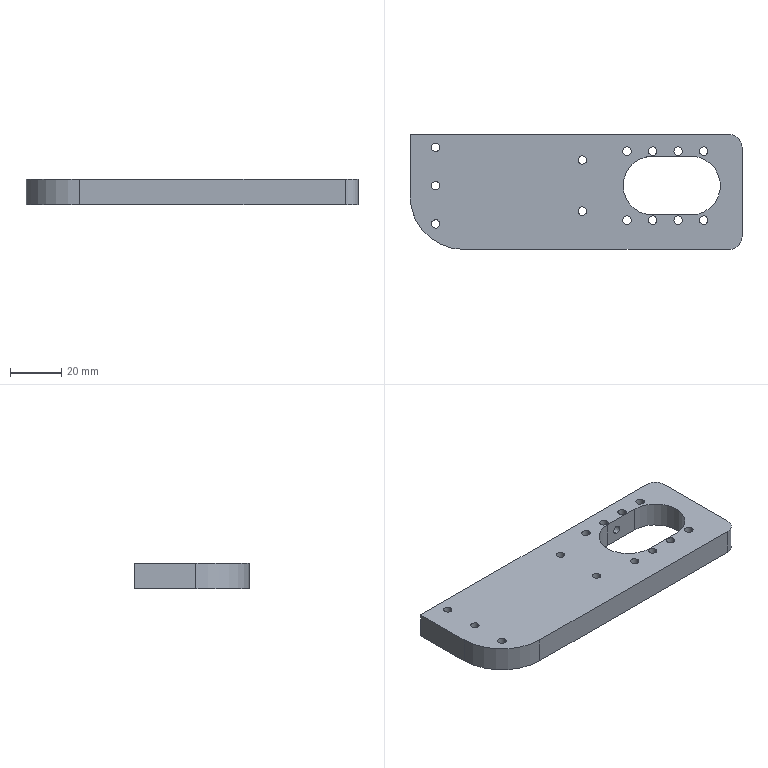Part | STEP file | 08-21 left conveyor adapter plate | 1 solid | 54 faces | box 130 x 45 x 10 mm | volume 48353 mm3 | cylinder 40 | plane 8 | cone 6 | commonest cylinder face diameters 3.3 x34 23 x3 10 x2 42 x1